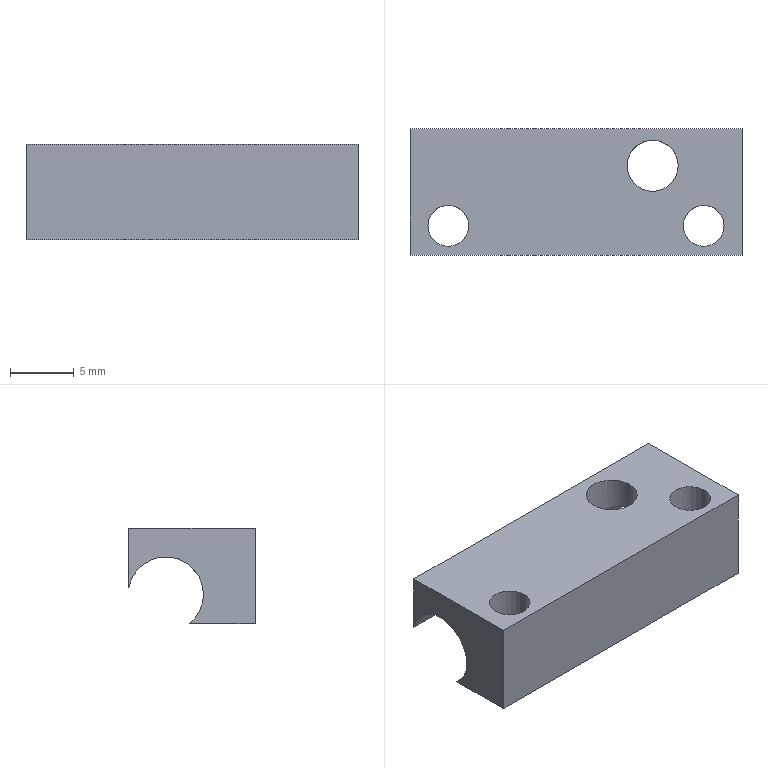Part | NX | 1 solid | 15 faces | box 26 x 9.9 x 7.5 mm | volume 1095 mm3 | cylinder 9 | plane 6 | commonest cylinder face diameters 3.2 x4 4 x3 5.9 x2
STEP:
#1=CARTESIAN_POINT('',(0.,5.153,-7.5));
#2=VERTEX_POINT('',#1);
#3=CARTESIAN_POINT('',(0.,4.05,-5.2));
#4=VERTEX_POINT('',#3);
#5=CARTESIAN_POINT('',(0.,7.,-5.2));
#6=DIRECTION('',(-1.,0.,0.));
#7=DIRECTION('',(0.,-1.,0.));
#8=AXIS2_PLACEMENT_3D('',#5,#6,#7);
#9=CIRCLE('',#8,2.95);
#10=EDGE_CURVE('',#2,#4,#9,.T.);
#11=ORIENTED_EDGE('',*,*,#10,.F.);
#12=CARTESIAN_POINT('',(0.,0.,-7.5));
#13=VERTEX_POINT('',#12);
#14=CARTESIAN_POINT('',(0.,5.153,-7.5));
#15=DIRECTION('',(0.,-1.,0.));
#16=VECTOR('',#15,1000.);
#17=LINE('',#14,#16);
#18=EDGE_CURVE('',#2,#13,#17,.T.);
#19=ORIENTED_EDGE('',*,*,#18,.T.);
#20=CARTESIAN_POINT('',(0.,0.,0.));
#21=VERTEX_POINT('',#20);
#22=CARTESIAN_POINT('',(0.,0.,-7.5));
#23=DIRECTION('',(0.,0.,1.));
#24=VECTOR('',#23,1000.);
#25=LINE('',#22,#24);
#26=EDGE_CURVE('',#13,#21,#25,.T.);
#27=ORIENTED_EDGE('',*,*,#26,.T.);
#28=CARTESIAN_POINT('',(0.,9.9,0.));
#29=VERTEX_POINT('',#28);
#30=CARTESIAN_POINT('',(0.,0.,0.));
#31=DIRECTION('',(0.,1.,0.));
#32=VECTOR('',#31,1000.);
#33=LINE('',#30,#32);
#34=EDGE_CURVE('',#21,#29,#33,.T.);
#35=ORIENTED_EDGE('',*,*,#34,.T.);
#36=CARTESIAN_POINT('',(0.,9.9,-4.659));
#37=VERTEX_POINT('',#36);
#38=CARTESIAN_POINT('',(0.,9.9,0.));
#39=DIRECTION('',(0.,0.,-1.));
#40=VECTOR('',#39,1000.);
#41=LINE('',#38,#40);
#42=EDGE_CURVE('',#29,#37,#41,.T.);
#43=ORIENTED_EDGE('',*,*,#42,.T.);
#44=CARTESIAN_POINT('',(0.,7.,-5.2));
#45=DIRECTION('',(-1.,0.,0.));
#46=DIRECTION('',(0.,-1.,0.));
#47=AXIS2_PLACEMENT_3D('',#44,#45,#46);
#48=CIRCLE('',#47,2.95);
#49=EDGE_CURVE('',#4,#37,#48,.T.);
#50=ORIENTED_EDGE('',*,*,#49,.F.);
#51=EDGE_LOOP('',(#11,#19,#27,#35,#43,#50));
#52=FACE_BOUND('',#51,.T.);
#53=CARTESIAN_POINT('',(0.,0.,0.));
#54=DIRECTION('',(1.,0.,0.));
#55=DIRECTION('',(0.,1.,0.));
#56=AXIS2_PLACEMENT_3D('',#53,#54,#55);
#57=PLANE('',#56);
#58=ADVANCED_FACE('',(#52),#57,.F.);
#59=CARTESIAN_POINT('',(17.,7.,-2.25));
#60=VERTEX_POINT('',#59);
#61=CARTESIAN_POINT('',(21.,7.,-2.25));
#62=VERTEX_POINT('',#61);
#63=CARTESIAN_POINT('',(17.,7.,-2.25));
#64=CARTESIAN_POINT('',(17.,7.06,-2.25));
#65=CARTESIAN_POINT('',(17.005,7.179,-2.254));
#66=CARTESIAN_POINT('',(17.03,7.358,-2.27));
#67=CARTESIAN_POINT('',(17.071,7.537,-2.297));
#68=CARTESIAN_POINT('',(17.129,7.715,-2.336));
#69=CARTESIAN_POINT('',(17.206,7.891,-2.386));
#70=CARTESIAN_POINT('',(17.302,8.064,-2.446));
#71=CARTESIAN_POINT('',(17.419,8.231,-2.517));
#72=CARTESIAN_POINT('',(17.556,8.389,-2.595));
#73=CARTESIAN_POINT('',(17.71,8.534,-2.678));
#74=CARTESIAN_POINT('',(17.879,8.661,-2.761));
#75=CARTESIAN_POINT('',(18.056,8.767,-2.837));
#76=CARTESIAN_POINT('',(18.235,8.851,-2.902));
#77=CARTESIAN_POINT('',(18.411,8.914,-2.955));
#78=CARTESIAN_POINT('',(18.583,8.959,-2.994));
#79=CARTESIAN_POINT('',(18.752,8.987,-3.019));
#80=CARTESIAN_POINT('',(18.917,9.001,-3.032));
#81=CARTESIAN_POINT('',(19.082,9.001,-3.032));
#82=CARTESIAN_POINT('',(19.248,8.987,-3.019));
#83=CARTESIAN_POINT('',(19.416,8.959,-2.994));
#84=CARTESIAN_POINT('',(19.588,8.914,-2.955));
#85=CARTESIAN_POINT('',(19.765,8.851,-2.903));
#86=CARTESIAN_POINT('',(19.943,8.767,-2.837));
#87=CARTESIAN_POINT('',(20.121,8.661,-2.761));
#88=CARTESIAN_POINT('',(20.289,8.534,-2.679));
#89=CARTESIAN_POINT('',(20.444,8.389,-2.595));
#90=CARTESIAN_POINT('',(20.581,8.231,-2.517));
#91=CARTESIAN_POINT('',(20.698,8.064,-2.446));
#92=CARTESIAN_POINT('',(20.794,7.891,-2.386));
#93=CARTESIAN_POINT('',(20.871,7.715,-2.336));
#94=CARTESIAN_POINT('',(20.929,7.537,-2.297));
#95=CARTESIAN_POINT('',(20.97,7.358,-2.27));
#96=CARTESIAN_POINT('',(20.995,7.179,-2.254));
#97=CARTESIAN_POINT('',(21.,7.06,-2.25));
#98=CARTESIAN_POINT('',(21.,7.,-2.25));
#99=B_SPLINE_CURVE_WITH_KNOTS('',3,(#63,#64,#65,#66,#67,#68,#69,#70,#71,#72,#73,#74,#75,#76,#77,#78,#79,#80,#81,#82,#83,#84,#85,#86,#87,#88,#89,#90,#91,#92,#93,#94,#95,#96,#97,#98),.UNSPECIFIED.,.F.,.F.,(4,1,1,1,1,1,1,1,1,1,1,1,1,1,1,1,1,1,1,1,1,1,1,1,1,1,1,1,1,1,1,1,1,4),(0.,0.0303,0.06061,0.09091,0.1212,0.1515,0.1818,0.2121,0.2424,0.2727,0.303,0.3333,0.3636,0.3939,0.4242,0.4545,0.4848,0.5152,0.5455,0.5758,0.6061,0.6364,0.6667,0.697,0.7273,0.7576,0.7879,0.8182,0.8485,0.8788,0.9091,0.9394,0.9697,1.),.UNSPECIFIED.);
#100=EDGE_CURVE('',#60,#62,#99,.T.);
#101=ORIENTED_EDGE('',*,*,#100,.F.);
#102=CARTESIAN_POINT('',(17.,7.,-2.25));
#103=CARTESIAN_POINT('',(17.,6.748,-2.25));
#104=CARTESIAN_POINT('',(17.086,6.264,-2.308));
#105=CARTESIAN_POINT('',(17.543,5.532,-2.607));
#106=CARTESIAN_POINT('',(18.316,5.064,-2.965));
#107=CARTESIAN_POINT('',(19.,4.968,-3.065));
#108=CARTESIAN_POINT('',(19.686,5.065,-2.964));
#109=CARTESIAN_POINT('',(20.457,5.532,-2.607));
#110=CARTESIAN_POINT('',(20.914,6.265,-2.308));
#111=CARTESIAN_POINT('',(21.,6.748,-2.25));
#112=CARTESIAN_POINT('',(21.,7.,-2.25));
#113=B_SPLINE_CURVE_WITH_KNOTS('',3,(#102,#103,#104,#105,#106,#107,#108,#109,#110,#111,#112),.UNSPECIFIED.,.F.,.F.,(4,1,1,1,1,1,1,1,4),(0.,0.125,0.25,0.375,0.5,0.625,0.75,0.875,1.),.UNSPECIFIED.);
#114=EDGE_CURVE('',#62,#60,#113,.F.);
#115=ORIENTED_EDGE('',*,*,#114,.F.);
#116=EDGE_LOOP('',(#101,#115));
#117=FACE_BOUND('',#116,.T.);
#118=CARTESIAN_POINT('',(26.,4.05,-5.2));
#119=VERTEX_POINT('',#118);
#120=CARTESIAN_POINT('',(26.,4.05,-5.2));
#121=DIRECTION('',(1.,0.,0.));
#122=VECTOR('',#121,1000.);
#123=LINE('',#120,#122);
#124=EDGE_CURVE('',#4,#119,#123,.T.);
#125=ORIENTED_EDGE('',*,*,#124,.F.);
#126=ORIENTED_EDGE('',*,*,#49,.T.);
#127=CARTESIAN_POINT('',(26.,9.9,-4.659));
#128=VERTEX_POINT('',#127);
#129=CARTESIAN_POINT('',(26.,9.9,-4.659));
#130=DIRECTION('',(-1.,0.,0.));
#131=VECTOR('',#130,1000.);
#132=LINE('',#129,#131);
#133=EDGE_CURVE('',#128,#37,#132,.T.);
#134=ORIENTED_EDGE('',*,*,#133,.F.);
#135=CARTESIAN_POINT('',(26.,7.,-5.2));
#136=DIRECTION('',(1.,0.,0.));
#137=DIRECTION('',(0.,0.9831,0.1833));
#138=AXIS2_PLACEMENT_3D('',#135,#136,#137);
#139=CIRCLE('',#138,2.95);
#140=EDGE_CURVE('',#128,#119,#139,.T.);
#141=ORIENTED_EDGE('',*,*,#140,.T.);
#142=EDGE_LOOP('',(#125,#126,#134,#141));
#143=FACE_BOUND('',#142,.T.);
#144=CARTESIAN_POINT('',(26.,7.,-5.2));
#145=DIRECTION('',(1.,0.,0.));
#146=DIRECTION('',(0.,-1.,0.));
#147=AXIS2_PLACEMENT_3D('',#144,#145,#146);
#148=CYLINDRICAL_SURFACE('',#147,2.95);
#149=ADVANCED_FACE('',(#117,#143),#148,.F.);
#150=CARTESIAN_POINT('',(19.766,5.153,-7.5));
#151=VERTEX_POINT('',#150);
#152=CARTESIAN_POINT('',(18.234,5.153,-7.5));
#153=VERTEX_POINT('',#152);
#154=CARTESIAN_POINT('',(19.,7.,-7.5));
#155=DIRECTION('',(0.,0.,-1.));
#156=DIRECTION('',(0.3832,-0.9236,0.));
#157=AXIS2_PLACEMENT_3D('',#154,#155,#156);
#158=CIRCLE('',#157,2.);
#159=EDGE_CURVE('',#151,#153,#158,.T.);
#160=ORIENTED_EDGE('',*,*,#159,.T.);
#161=CARTESIAN_POINT('',(18.234,5.153,-7.5));
#162=CARTESIAN_POINT('',(18.746,4.94,-7.329));
#163=CARTESIAN_POINT('',(19.254,4.94,-7.329));
#164=CARTESIAN_POINT('',(19.766,5.153,-7.5));
#165=B_SPLINE_CURVE_WITH_KNOTS('',3,(#161,#162,#163,#164),.UNSPECIFIED.,.F.,.F.,(4,4),(0.,1.),.UNSPECIFIED.);
#166=EDGE_CURVE('',#153,#151,#165,.T.);
#167=ORIENTED_EDGE('',*,*,#166,.T.);
#168=EDGE_LOOP('',(#160,#167));
#169=FACE_BOUND('',#168,.T.);
#170=CARTESIAN_POINT('',(19.,7.,0.));
#171=DIRECTION('',(0.,0.,-1.));
#172=DIRECTION('',(-1.,0.,0.));
#173=AXIS2_PLACEMENT_3D('',#170,#171,#172);
#174=CYLINDRICAL_SURFACE('',#173,2.);
#175=ADVANCED_FACE('',(#169),#174,.F.);
#176=ORIENTED_EDGE('',*,*,#159,.F.);
#177=CARTESIAN_POINT('',(26.,5.153,-7.5));
#178=VERTEX_POINT('',#177);
#179=CARTESIAN_POINT('',(19.766,5.153,-7.5));
#180=DIRECTION('',(1.,0.,0.));
#181=VECTOR('',#180,1000.);
#182=LINE('',#179,#181);
#183=EDGE_CURVE('',#151,#178,#182,.T.);
#184=ORIENTED_EDGE('',*,*,#183,.T.);
#185=CARTESIAN_POINT('',(26.,0.,-7.5));
#186=VERTEX_POINT('',#185);
#187=CARTESIAN_POINT('',(26.,5.153,-7.5));
#188=DIRECTION('',(0.,-1.,0.));
#189=VECTOR('',#188,1000.);
#190=LINE('',#187,#189);
#191=EDGE_CURVE('',#178,#186,#190,.T.);
#192=ORIENTED_EDGE('',*,*,#191,.T.);
#193=CARTESIAN_POINT('',(26.,0.,-7.5));
#194=DIRECTION('',(-1.,0.,0.));
#195=VECTOR('',#194,1000.);
#196=LINE('',#193,#195);
#197=EDGE_CURVE('',#186,#13,#196,.T.);
#198=ORIENTED_EDGE('',*,*,#197,.T.);
#199=ORIENTED_EDGE('',*,*,#18,.F.);
#200=CARTESIAN_POINT('',(0.,5.153,-7.5));
#201=DIRECTION('',(1.,0.,0.));
#202=VECTOR('',#201,1000.);
#203=LINE('',#200,#202);
#204=EDGE_CURVE('',#2,#153,#203,.T.);
#205=ORIENTED_EDGE('',*,*,#204,.T.);
#206=EDGE_LOOP('',(#176,#184,#192,#198,#199,#205));
#207=FACE_BOUND('',#206,.T.);
#208=CARTESIAN_POINT('',(4.6,2.3,-7.5));
#209=VERTEX_POINT('',#208);
#210=CARTESIAN_POINT('',(1.4,2.3,-7.5));
#211=VERTEX_POINT('',#210);
#212=CARTESIAN_POINT('',(3.,2.3,-7.5));
#213=DIRECTION('',(0.,0.,-1.));
#214=DIRECTION('',(1.,0.,0.));
#215=AXIS2_PLACEMENT_3D('',#212,#213,#214);
#216=CIRCLE('',#215,1.6);
#217=EDGE_CURVE('',#209,#211,#216,.T.);
#218=ORIENTED_EDGE('',*,*,#217,.F.);
#219=CARTESIAN_POINT('',(3.,2.3,-7.5));
#220=DIRECTION('',(0.,0.,-1.));
#221=DIRECTION('',(1.,0.,0.));
#222=AXIS2_PLACEMENT_3D('',#219,#220,#221);
#223=CIRCLE('',#222,1.6);
#224=EDGE_CURVE('',#211,#209,#223,.T.);
#225=ORIENTED_EDGE('',*,*,#224,.F.);
#226=EDGE_LOOP('',(#218,#225));
#227=FACE_BOUND('',#226,.T.);
#228=CARTESIAN_POINT('',(24.6,2.3,-7.5));
#229=VERTEX_POINT('',#228);
#230=CARTESIAN_POINT('',(21.4,2.3,-7.5));
#231=VERTEX_POINT('',#230);
#232=CARTESIAN_POINT('',(23.,2.3,-7.5));
#233=DIRECTION('',(0.,0.,-1.));
#234=DIRECTION('',(1.,0.,0.));
#235=AXIS2_PLACEMENT_3D('',#232,#233,#234);
#236=CIRCLE('',#235,1.6);
#237=EDGE_CURVE('',#229,#231,#236,.T.);
#238=ORIENTED_EDGE('',*,*,#237,.F.);
#239=CARTESIAN_POINT('',(23.,2.3,-7.5));
#240=DIRECTION('',(0.,0.,-1.));
#241=DIRECTION('',(1.,0.,0.));
#242=AXIS2_PLACEMENT_3D('',#239,#240,#241);
#243=CIRCLE('',#242,1.6);
#244=EDGE_CURVE('',#231,#229,#243,.T.);
#245=ORIENTED_EDGE('',*,*,#244,.F.);
#246=EDGE_LOOP('',(#238,#245));
#247=FACE_BOUND('',#246,.T.);
#248=CARTESIAN_POINT('',(0.,0.,-7.5));
#249=DIRECTION('',(0.,0.,-1.));
#250=DIRECTION('',(0.,-1.,0.));
#251=AXIS2_PLACEMENT_3D('',#248,#249,#250);
#252=PLANE('',#251);
#253=ADVANCED_FACE('',(#207,#227,#247),#252,.T.);
#254=ORIENTED_EDGE('',*,*,#26,.F.);
#255=ORIENTED_EDGE('',*,*,#197,.F.);
#256=CARTESIAN_POINT('',(26.,0.,0.));
#257=VERTEX_POINT('',#256);
#258=CARTESIAN_POINT('',(26.,0.,-7.5));
#259=DIRECTION('',(0.,0.,1.));
#260=VECTOR('',#259,1000.);
#261=LINE('',#258,#260);
#262=EDGE_CURVE('',#186,#257,#261,.T.);
#263=ORIENTED_EDGE('',*,*,#262,.T.);
#264=CARTESIAN_POINT('',(26.,0.,0.));
#265=DIRECTION('',(-1.,0.,0.));
#266=VECTOR('',#265,1000.);
#267=LINE('',#264,#266);
#268=EDGE_CURVE('',#257,#21,#267,.T.);
#269=ORIENTED_EDGE('',*,*,#268,.T.);
#270=EDGE_LOOP('',(#254,#255,#263,#269));
#271=FACE_BOUND('',#270,.T.);
#272=CARTESIAN_POINT('',(0.,0.,0.));
#273=DIRECTION('',(0.,-1.,0.));
#274=DIRECTION('',(0.,0.,-1.));
#275=AXIS2_PLACEMENT_3D('',#272,#273,#274);
#276=PLANE('',#275);
#277=ADVANCED_FACE('',(#271),#276,.T.);
#278=ORIENTED_EDGE('',*,*,#34,.F.);
#279=ORIENTED_EDGE('',*,*,#268,.F.);
#280=CARTESIAN_POINT('',(26.,9.9,0.));
#281=VERTEX_POINT('',#280);
#282=CARTESIAN_POINT('',(26.,0.,0.));
#283=DIRECTION('',(0.,1.,0.));
#284=VECTOR('',#283,1000.);
#285=LINE('',#282,#284);
#286=EDGE_CURVE('',#257,#281,#285,.T.);
#287=ORIENTED_EDGE('',*,*,#286,.T.);
#288=CARTESIAN_POINT('',(26.,9.9,0.));
#289=DIRECTION('',(-1.,0.,0.));
#290=VECTOR('',#289,1000.);
#291=LINE('',#288,#290);
#292=EDGE_CURVE('',#281,#29,#291,.T.);
#293=ORIENTED_EDGE('',*,*,#292,.T.);
#294=EDGE_LOOP('',(#278,#279,#287,#293));
#295=FACE_BOUND('',#294,.T.);
#296=CARTESIAN_POINT('',(4.6,2.3,0.));
#297=VERTEX_POINT('',#296);
#298=CARTESIAN_POINT('',(1.4,2.3,0.));
#299=VERTEX_POINT('',#298);
#300=CARTESIAN_POINT('',(3.,2.3,0.));
#301=DIRECTION('',(0.,0.,1.));
#302=DIRECTION('',(-1.,0.,0.));
#303=AXIS2_PLACEMENT_3D('',#300,#301,#302);
#304=CIRCLE('',#303,1.6);
#305=EDGE_CURVE('',#297,#299,#304,.T.);
#306=ORIENTED_EDGE('',*,*,#305,.F.);
#307=CARTESIAN_POINT('',(3.,2.3,0.));
#308=DIRECTION('',(0.,0.,1.));
#309=DIRECTION('',(-1.,0.,0.));
#310=AXIS2_PLACEMENT_3D('',#307,#308,#309);
#311=CIRCLE('',#310,1.6);
#312=EDGE_CURVE('',#299,#297,#311,.T.);
#313=ORIENTED_EDGE('',*,*,#312,.F.);
#314=EDGE_LOOP('',(#306,#313));
#315=FACE_BOUND('',#314,.T.);
#316=CARTESIAN_POINT('',(24.6,2.3,0.));
#317=VERTEX_POINT('',#316);
#318=CARTESIAN_POINT('',(21.4,2.3,0.));
#319=VERTEX_POINT('',#318);
#320=CARTESIAN_POINT('',(23.,2.3,0.));
#321=DIRECTION('',(0.,0.,1.));
#322=DIRECTION('',(-1.,0.,0.));
#323=AXIS2_PLACEMENT_3D('',#320,#321,#322);
#324=CIRCLE('',#323,1.6);
#325=EDGE_CURVE('',#317,#319,#324,.T.);
#326=ORIENTED_EDGE('',*,*,#325,.F.);
#327=CARTESIAN_POINT('',(23.,2.3,0.));
#328=DIRECTION('',(0.,0.,1.));
#329=DIRECTION('',(-1.,0.,0.));
#330=AXIS2_PLACEMENT_3D('',#327,#328,#329);
#331=CIRCLE('',#330,1.6);
#332=EDGE_CURVE('',#319,#317,#331,.T.);
#333=ORIENTED_EDGE('',*,*,#332,.F.);
#334=EDGE_LOOP('',(#326,#333));
#335=FACE_BOUND('',#334,.T.);
#336=CARTESIAN_POINT('',(21.,7.,0.));
#337=VERTEX_POINT('',#336);
#338=CARTESIAN_POINT('',(17.,7.,0.));
#339=VERTEX_POINT('',#338);
#340=CARTESIAN_POINT('',(19.,7.,0.));
#341=DIRECTION('',(0.,0.,1.));
#342=DIRECTION('',(-1.,0.,0.));
#343=AXIS2_PLACEMENT_3D('',#340,#341,#342);
#344=CIRCLE('',#343,2.);
#345=EDGE_CURVE('',#337,#339,#344,.T.);
#346=ORIENTED_EDGE('',*,*,#345,.F.);
#347=CARTESIAN_POINT('',(19.,7.,0.));
#348=DIRECTION('',(0.,0.,1.));
#349=DIRECTION('',(-1.,0.,0.));
#350=AXIS2_PLACEMENT_3D('',#347,#348,#349);
#351=CIRCLE('',#350,2.);
#352=EDGE_CURVE('',#339,#337,#351,.T.);
#353=ORIENTED_EDGE('',*,*,#352,.F.);
#354=EDGE_LOOP('',(#346,#353));
#355=FACE_BOUND('',#354,.T.);
#356=CARTESIAN_POINT('',(0.,9.9,0.));
#357=DIRECTION('',(0.,0.,1.));
#358=DIRECTION('',(1.,0.,0.));
#359=AXIS2_PLACEMENT_3D('',#356,#357,#358);
#360=PLANE('',#359);
#361=ADVANCED_FACE('',(#295,#315,#335,#355),#360,.T.);
#362=ORIENTED_EDGE('',*,*,#133,.T.);
#363=ORIENTED_EDGE('',*,*,#42,.F.);
#364=ORIENTED_EDGE('',*,*,#292,.F.);
#365=CARTESIAN_POINT('',(26.,9.9,0.));
#366=DIRECTION('',(0.,0.,-1.));
#367=VECTOR('',#366,1000.);
#368=LINE('',#365,#367);
#369=EDGE_CURVE('',#281,#128,#368,.T.);
#370=ORIENTED_EDGE('',*,*,#369,.T.);
#371=EDGE_LOOP('',(#362,#363,#364,#370));
#372=FACE_BOUND('',#371,.T.);
#373=CARTESIAN_POINT('',(0.,9.9,-7.5));
#374=DIRECTION('',(0.,1.,0.));
#375=DIRECTION('',(1.,0.,0.));
#376=AXIS2_PLACEMENT_3D('',#373,#374,#375);
#377=PLANE('',#376);
#378=ADVANCED_FACE('',(#372),#377,.T.);
#379=ORIENTED_EDGE('',*,*,#140,.F.);
#380=ORIENTED_EDGE('',*,*,#369,.F.);
#381=ORIENTED_EDGE('',*,*,#286,.F.);
#382=ORIENTED_EDGE('',*,*,#262,.F.);
#383=ORIENTED_EDGE('',*,*,#191,.F.);
#384=CARTESIAN_POINT('',(26.,7.,-5.2));
#385=DIRECTION('',(1.,0.,0.));
#386=DIRECTION('',(0.,0.9831,0.1833));
#387=AXIS2_PLACEMENT_3D('',#384,#385,#386);
#388=CIRCLE('',#387,2.95);
#389=EDGE_CURVE('',#119,#178,#388,.T.);
#390=ORIENTED_EDGE('',*,*,#389,.F.);
#391=EDGE_LOOP('',(#379,#380,#381,#382,#383,#390));
#392=FACE_BOUND('',#391,.T.);
#393=CARTESIAN_POINT('',(26.,0.,0.));
#394=DIRECTION('',(1.,0.,0.));
#395=DIRECTION('',(0.,1.,0.));
#396=AXIS2_PLACEMENT_3D('',#393,#394,#395);
#397=PLANE('',#396);
#398=ADVANCED_FACE('',(#392),#397,.T.);
#399=ORIENTED_EDGE('',*,*,#217,.T.);
#400=CARTESIAN_POINT('',(1.4,2.3,0.));
#401=DIRECTION('',(0.,0.,-1.));
#402=VECTOR('',#401,1000.);
#403=LINE('',#400,#402);
#404=EDGE_CURVE('',#211,#299,#403,.F.);
#405=ORIENTED_EDGE('',*,*,#404,.T.);
#406=ORIENTED_EDGE('',*,*,#312,.T.);
#407=CARTESIAN_POINT('',(4.6,2.3,0.));
#408=DIRECTION('',(0.,0.,-1.));
#409=VECTOR('',#408,1000.);
#410=LINE('',#407,#409);
#411=EDGE_CURVE('',#209,#297,#410,.F.);
#412=ORIENTED_EDGE('',*,*,#411,.F.);
#413=EDGE_LOOP('',(#399,#405,#406,#412));
#414=FACE_BOUND('',#413,.T.);
#415=CARTESIAN_POINT('',(3.,2.3,0.));
#416=DIRECTION('',(0.,0.,-1.));
#417=DIRECTION('',(-1.,0.,0.));
#418=AXIS2_PLACEMENT_3D('',#415,#416,#417);
#419=CYLINDRICAL_SURFACE('',#418,1.6);
#420=ADVANCED_FACE('',(#414),#419,.F.);
#421=ORIENTED_EDGE('',*,*,#100,.T.);
#422=CARTESIAN_POINT('',(21.,7.,0.));
#423=DIRECTION('',(0.,0.,-1.));
#424=VECTOR('',#423,1000.);
#425=LINE('',#422,#424);
#426=EDGE_CURVE('',#62,#337,#425,.F.);
#427=ORIENTED_EDGE('',*,*,#426,.T.);
#428=ORIENTED_EDGE('',*,*,#345,.T.);
#429=CARTESIAN_POINT('',(17.,7.,0.));
#430=DIRECTION('',(0.,0.,-1.));
#431=VECTOR('',#430,1000.);
#432=LINE('',#429,#431);
#433=EDGE_CURVE('',#60,#339,#432,.F.);
#434=ORIENTED_EDGE('',*,*,#433,.F.);
#435=EDGE_LOOP('',(#421,#427,#428,#434));
#436=FACE_BOUND('',#435,.T.);
#437=CARTESIAN_POINT('',(19.,7.,0.));
#438=DIRECTION('',(0.,0.,-1.));
#439=DIRECTION('',(-1.,0.,0.));
#440=AXIS2_PLACEMENT_3D('',#437,#438,#439);
#441=CYLINDRICAL_SURFACE('',#440,2.);
#442=ADVANCED_FACE('',(#436),#441,.F.);
#443=ORIENTED_EDGE('',*,*,#325,.T.);
#444=CARTESIAN_POINT('',(21.4,2.3,0.));
#445=DIRECTION('',(0.,0.,-1.));
#446=VECTOR('',#445,1000.);
#447=LINE('',#444,#446);
#448=EDGE_CURVE('',#231,#319,#447,.F.);
#449=ORIENTED_EDGE('',*,*,#448,.F.);
#450=ORIENTED_EDGE('',*,*,#244,.T.);
#451=CARTESIAN_POINT('',(24.6,2.3,0.));
#452=DIRECTION('',(0.,0.,-1.));
#453=VECTOR('',#452,1000.);
#454=LINE('',#451,#453);
#455=EDGE_CURVE('',#229,#317,#454,.F.);
#456=ORIENTED_EDGE('',*,*,#455,.T.);
#457=EDGE_LOOP('',(#443,#449,#450,#456));
#458=FACE_BOUND('',#457,.T.);
#459=CARTESIAN_POINT('',(23.,2.3,0.));
#460=DIRECTION('',(0.,0.,-1.));
#461=DIRECTION('',(-1.,0.,0.));
#462=AXIS2_PLACEMENT_3D('',#459,#460,#461);
#463=CYLINDRICAL_SURFACE('',#462,1.6);
#464=ADVANCED_FACE('',(#458),#463,.F.);
#465=ORIENTED_EDGE('',*,*,#433,.T.);
#466=ORIENTED_EDGE('',*,*,#352,.T.);
#467=ORIENTED_EDGE('',*,*,#426,.F.);
#468=ORIENTED_EDGE('',*,*,#114,.T.);
#469=EDGE_LOOP('',(#465,#466,#467,#468));
#470=FACE_BOUND('',#469,.T.);
#471=CARTESIAN_POINT('',(19.,7.,0.));
#472=DIRECTION('',(0.,0.,-1.));
#473=DIRECTION('',(-1.,0.,0.));
#474=AXIS2_PLACEMENT_3D('',#471,#472,#473);
#475=CYLINDRICAL_SURFACE('',#474,2.);
#476=ADVANCED_FACE('',(#470),#475,.F.);
#477=ORIENTED_EDGE('',*,*,#305,.T.);
#478=ORIENTED_EDGE('',*,*,#404,.F.);
#479=ORIENTED_EDGE('',*,*,#224,.T.);
#480=ORIENTED_EDGE('',*,*,#411,.T.);
#481=EDGE_LOOP('',(#477,#478,#479,#480));
#482=FACE_BOUND('',#481,.T.);
#483=CARTESIAN_POINT('',(3.,2.3,0.));
#484=DIRECTION('',(0.,0.,-1.));
#485=DIRECTION('',(-1.,0.,0.));
#486=AXIS2_PLACEMENT_3D('',#483,#484,#485);
#487=CYLINDRICAL_SURFACE('',#486,1.6);
#488=ADVANCED_FACE('',(#482),#487,.F.);
#489=ORIENTED_EDGE('',*,*,#237,.T.);
#490=ORIENTED_EDGE('',*,*,#448,.T.);
#491=ORIENTED_EDGE('',*,*,#332,.T.);
#492=ORIENTED_EDGE('',*,*,#455,.F.);
#493=EDGE_LOOP('',(#489,#490,#491,#492));
#494=FACE_BOUND('',#493,.T.);
#495=CARTESIAN_POINT('',(23.,2.3,0.));
#496=DIRECTION('',(0.,0.,-1.));
#497=DIRECTION('',(-1.,0.,0.));
#498=AXIS2_PLACEMENT_3D('',#495,#496,#497);
#499=CYLINDRICAL_SURFACE('',#498,1.6);
#500=ADVANCED_FACE('',(#494),#499,.F.);
#501=ORIENTED_EDGE('',*,*,#10,.T.);
#502=ORIENTED_EDGE('',*,*,#124,.T.);
#503=ORIENTED_EDGE('',*,*,#389,.T.);
#504=ORIENTED_EDGE('',*,*,#183,.F.);
#505=ORIENTED_EDGE('',*,*,#166,.F.);
#506=ORIENTED_EDGE('',*,*,#204,.F.);
#507=EDGE_LOOP('',(#501,#502,#503,#504,#505,#506));
#508=FACE_BOUND('',#507,.T.);
#509=CARTESIAN_POINT('',(26.,7.,-5.2));
#510=DIRECTION('',(1.,0.,0.));
#511=DIRECTION('',(0.,-1.,0.));
#512=AXIS2_PLACEMENT_3D('',#509,#510,#511);
#513=CYLINDRICAL_SURFACE('',#512,2.95);
#514=ADVANCED_FACE('',(#508),#513,.F.);
#515=CLOSED_SHELL('',(#58,#149,#175,#253,#277,#361,#378,#398,#420,#442,#464,#476,#488,#500,#514));
#516=MANIFOLD_SOLID_BREP('',#515);
#517=(LENGTH_UNIT()NAMED_UNIT(*)SI_UNIT(.MILLI.,.METRE.));
#518=UNCERTAINTY_MEASURE_WITH_UNIT(LENGTH_MEASURE(0.0508),#517,'','');
#519=(NAMED_UNIT(*)PLANE_ANGLE_UNIT()SI_UNIT($,.RADIAN.));
#520=(NAMED_UNIT(*)SI_UNIT($,.STERADIAN.)SOLID_ANGLE_UNIT());
#521=(GEOMETRIC_REPRESENTATION_CONTEXT(3)GLOBAL_UNCERTAINTY_ASSIGNED_CONTEXT((#518))GLOBAL_UNIT_ASSIGNED_CONTEXT((#517,#519,#520))REPRESENTATION_CONTEXT('',''));
#522=ADVANCED_BREP_SHAPE_REPRESENTATION('',(#516),#521);